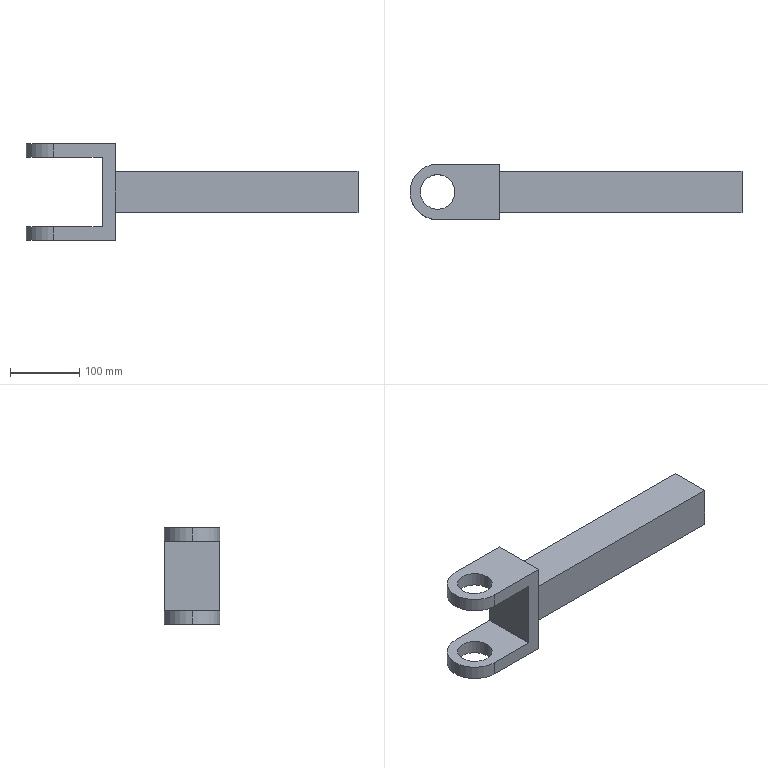Part | SolidWorks | 1 solid | 21 faces | box 480 x 80 x 140 mm | volume 1729991 mm3 | plane 13 | cylinder 8 | commonest cylinder face diameters 50 x4 80 x4
STEP:
#1=CARTESIAN_POINT('',(25.,0.,-50.));
#2=VERTEX_POINT('',#1);
#3=CARTESIAN_POINT('',(-25.,0.,-50.));
#4=VERTEX_POINT('',#3);
#5=CARTESIAN_POINT('',(0.,0.,-50.));
#6=DIRECTION('',(0.,0.,-1.));
#7=DIRECTION('',(-1.,0.,0.));
#8=AXIS2_PLACEMENT_3D('',#5,#6,#7);
#9=CIRCLE('',#8,25.);
#10=EDGE_CURVE('',#2,#4,#9,.T.);
#11=ORIENTED_EDGE('',*,*,#10,.F.);
#12=CARTESIAN_POINT('',(25.,0.,-70.));
#13=VERTEX_POINT('',#12);
#14=CARTESIAN_POINT('',(25.,0.,70.));
#15=DIRECTION('',(0.,0.,-1.));
#16=VECTOR('',#15,1000.);
#17=LINE('',#14,#16);
#18=EDGE_CURVE('',#2,#13,#17,.T.);
#19=ORIENTED_EDGE('',*,*,#18,.T.);
#20=CARTESIAN_POINT('',(-25.,0.,-70.));
#21=VERTEX_POINT('',#20);
#22=CARTESIAN_POINT('',(0.,0.,-70.));
#23=DIRECTION('',(0.,0.,1.));
#24=DIRECTION('',(1.,0.,0.));
#25=AXIS2_PLACEMENT_3D('',#22,#23,#24);
#26=CIRCLE('',#25,25.);
#27=EDGE_CURVE('',#21,#13,#26,.T.);
#28=ORIENTED_EDGE('',*,*,#27,.F.);
#29=CARTESIAN_POINT('',(-25.,0.,70.));
#30=DIRECTION('',(0.,0.,-1.));
#31=VECTOR('',#30,1000.);
#32=LINE('',#29,#31);
#33=EDGE_CURVE('',#4,#21,#32,.T.);
#34=ORIENTED_EDGE('',*,*,#33,.F.);
#35=EDGE_LOOP('',(#11,#19,#28,#34));
#36=FACE_OUTER_BOUND('',#35,.T.);
#37=CARTESIAN_POINT('',(0.,0.,70.));
#38=DIRECTION('',(0.,0.,-1.));
#39=DIRECTION('',(-1.,0.,0.));
#40=AXIS2_PLACEMENT_3D('',#37,#38,#39);
#41=CYLINDRICAL_SURFACE('',#40,25.);
#42=ADVANCED_FACE('',(#36),#41,.F.);
#43=CARTESIAN_POINT('',(0.,-40.,-50.));
#44=VERTEX_POINT('',#43);
#45=CARTESIAN_POINT('',(-40.,0.,-50.));
#46=VERTEX_POINT('',#45);
#47=CARTESIAN_POINT('',(0.,0.,-50.));
#48=DIRECTION('',(0.,0.,-1.));
#49=DIRECTION('',(-1.,0.,0.));
#50=AXIS2_PLACEMENT_3D('',#47,#48,#49);
#51=CIRCLE('',#50,40.);
#52=EDGE_CURVE('',#44,#46,#51,.T.);
#53=ORIENTED_EDGE('',*,*,#52,.T.);
#54=CARTESIAN_POINT('',(-40.,0.,-70.));
#55=VERTEX_POINT('',#54);
#56=CARTESIAN_POINT('',(-40.,0.,70.));
#57=DIRECTION('',(0.,0.,-1.));
#58=VECTOR('',#57,1000.);
#59=LINE('',#56,#58);
#60=EDGE_CURVE('',#46,#55,#59,.T.);
#61=ORIENTED_EDGE('',*,*,#60,.T.);
#62=CARTESIAN_POINT('',(0.,-40.,-70.));
#63=VERTEX_POINT('',#62);
#64=CARTESIAN_POINT('',(0.,0.,-70.));
#65=DIRECTION('',(0.,0.,1.));
#66=DIRECTION('',(1.,0.,0.));
#67=AXIS2_PLACEMENT_3D('',#64,#65,#66);
#68=CIRCLE('',#67,40.);
#69=EDGE_CURVE('',#55,#63,#68,.T.);
#70=ORIENTED_EDGE('',*,*,#69,.T.);
#71=CARTESIAN_POINT('',(0.,-40.,70.));
#72=DIRECTION('',(0.,0.,-1.));
#73=VECTOR('',#72,1000.);
#74=LINE('',#71,#73);
#75=EDGE_CURVE('',#44,#63,#74,.T.);
#76=ORIENTED_EDGE('',*,*,#75,.F.);
#77=EDGE_LOOP('',(#53,#61,#70,#76));
#78=FACE_OUTER_BOUND('',#77,.T.);
#79=CARTESIAN_POINT('',(0.,0.,70.));
#80=DIRECTION('',(0.,0.,-1.));
#81=DIRECTION('',(-1.,0.,0.));
#82=AXIS2_PLACEMENT_3D('',#79,#80,#81);
#83=CYLINDRICAL_SURFACE('',#82,40.);
#84=ADVANCED_FACE('',(#78),#83,.T.);
#85=CARTESIAN_POINT('',(-25.,0.,70.));
#86=VERTEX_POINT('',#85);
#87=CARTESIAN_POINT('',(25.,0.,70.));
#88=VERTEX_POINT('',#87);
#89=CARTESIAN_POINT('',(0.,0.,70.));
#90=DIRECTION('',(0.,0.,1.));
#91=DIRECTION('',(1.,0.,0.));
#92=AXIS2_PLACEMENT_3D('',#89,#90,#91);
#93=CIRCLE('',#92,25.);
#94=EDGE_CURVE('',#86,#88,#93,.T.);
#95=ORIENTED_EDGE('',*,*,#94,.T.);
#96=CARTESIAN_POINT('',(25.,0.,50.));
#97=VERTEX_POINT('',#96);
#98=CARTESIAN_POINT('',(25.,0.,70.));
#99=DIRECTION('',(0.,0.,-1.));
#100=VECTOR('',#99,1000.);
#101=LINE('',#98,#100);
#102=EDGE_CURVE('',#88,#97,#101,.T.);
#103=ORIENTED_EDGE('',*,*,#102,.T.);
#104=CARTESIAN_POINT('',(-25.,0.,50.));
#105=VERTEX_POINT('',#104);
#106=CARTESIAN_POINT('',(0.,0.,50.));
#107=DIRECTION('',(0.,0.,1.));
#108=DIRECTION('',(1.,0.,0.));
#109=AXIS2_PLACEMENT_3D('',#106,#107,#108);
#110=CIRCLE('',#109,25.);
#111=EDGE_CURVE('',#105,#97,#110,.T.);
#112=ORIENTED_EDGE('',*,*,#111,.F.);
#113=CARTESIAN_POINT('',(-25.,0.,70.));
#114=DIRECTION('',(0.,0.,-1.));
#115=VECTOR('',#114,1000.);
#116=LINE('',#113,#115);
#117=EDGE_CURVE('',#86,#105,#116,.T.);
#118=ORIENTED_EDGE('',*,*,#117,.F.);
#119=EDGE_LOOP('',(#95,#103,#112,#118));
#120=FACE_OUTER_BOUND('',#119,.T.);
#121=CARTESIAN_POINT('',(0.,0.,70.));
#122=DIRECTION('',(0.,0.,-1.));
#123=DIRECTION('',(-1.,0.,0.));
#124=AXIS2_PLACEMENT_3D('',#121,#122,#123);
#125=CYLINDRICAL_SURFACE('',#124,25.);
#126=ADVANCED_FACE('',(#120),#125,.F.);
#127=CARTESIAN_POINT('',(-40.,0.,70.));
#128=VERTEX_POINT('',#127);
#129=CARTESIAN_POINT('',(0.,-40.,70.));
#130=VERTEX_POINT('',#129);
#131=CARTESIAN_POINT('',(0.,0.,70.));
#132=DIRECTION('',(0.,0.,1.));
#133=DIRECTION('',(1.,0.,0.));
#134=AXIS2_PLACEMENT_3D('',#131,#132,#133);
#135=CIRCLE('',#134,40.);
#136=EDGE_CURVE('',#128,#130,#135,.T.);
#137=ORIENTED_EDGE('',*,*,#136,.F.);
#138=CARTESIAN_POINT('',(-40.,0.,50.));
#139=VERTEX_POINT('',#138);
#140=CARTESIAN_POINT('',(-40.,0.,70.));
#141=DIRECTION('',(0.,0.,-1.));
#142=VECTOR('',#141,1000.);
#143=LINE('',#140,#142);
#144=EDGE_CURVE('',#128,#139,#143,.T.);
#145=ORIENTED_EDGE('',*,*,#144,.T.);
#146=CARTESIAN_POINT('',(0.,-40.,50.));
#147=VERTEX_POINT('',#146);
#148=CARTESIAN_POINT('',(0.,0.,50.));
#149=DIRECTION('',(0.,0.,1.));
#150=DIRECTION('',(1.,0.,0.));
#151=AXIS2_PLACEMENT_3D('',#148,#149,#150);
#152=CIRCLE('',#151,40.);
#153=EDGE_CURVE('',#139,#147,#152,.T.);
#154=ORIENTED_EDGE('',*,*,#153,.T.);
#155=CARTESIAN_POINT('',(0.,-40.,70.));
#156=DIRECTION('',(0.,0.,-1.));
#157=VECTOR('',#156,1000.);
#158=LINE('',#155,#157);
#159=EDGE_CURVE('',#130,#147,#158,.T.);
#160=ORIENTED_EDGE('',*,*,#159,.F.);
#161=EDGE_LOOP('',(#137,#145,#154,#160));
#162=FACE_OUTER_BOUND('',#161,.T.);
#163=CARTESIAN_POINT('',(0.,0.,70.));
#164=DIRECTION('',(0.,0.,-1.));
#165=DIRECTION('',(-1.,0.,0.));
#166=AXIS2_PLACEMENT_3D('',#163,#164,#165);
#167=CYLINDRICAL_SURFACE('',#166,40.);
#168=ADVANCED_FACE('',(#162),#167,.T.);
#169=CARTESIAN_POINT('',(70.,-40.,-50.));
#170=VERTEX_POINT('',#169);
#171=CARTESIAN_POINT('',(70.,40.,-50.));
#172=VERTEX_POINT('',#171);
#173=CARTESIAN_POINT('',(70.,0.,-50.));
#174=DIRECTION('',(0.,1.,0.));
#175=VECTOR('',#174,1000.);
#176=LINE('',#173,#175);
#177=EDGE_CURVE('',#170,#172,#176,.T.);
#178=ORIENTED_EDGE('',*,*,#177,.F.);
#179=CARTESIAN_POINT('',(70.,-40.,50.));
#180=VERTEX_POINT('',#179);
#181=CARTESIAN_POINT('',(70.,-40.,70.));
#182=DIRECTION('',(0.,0.,-1.));
#183=VECTOR('',#182,1000.);
#184=LINE('',#181,#183);
#185=EDGE_CURVE('',#180,#170,#184,.T.);
#186=ORIENTED_EDGE('',*,*,#185,.F.);
#187=CARTESIAN_POINT('',(70.,40.,50.));
#188=VERTEX_POINT('',#187);
#189=CARTESIAN_POINT('',(70.,-100.,50.));
#190=DIRECTION('',(0.,1.,0.));
#191=VECTOR('',#190,1000.);
#192=LINE('',#189,#191);
#193=EDGE_CURVE('',#180,#188,#192,.T.);
#194=ORIENTED_EDGE('',*,*,#193,.T.);
#195=CARTESIAN_POINT('',(70.,40.,70.));
#196=DIRECTION('',(0.,0.,1.));
#197=VECTOR('',#196,1000.);
#198=LINE('',#195,#197);
#199=EDGE_CURVE('',#172,#188,#198,.T.);
#200=ORIENTED_EDGE('',*,*,#199,.F.);
#201=EDGE_LOOP('',(#178,#186,#194,#200));
#202=FACE_OUTER_BOUND('',#201,.T.);
#203=CARTESIAN_POINT('',(70.,0.,0.));
#204=DIRECTION('',(1.,0.,0.));
#205=DIRECTION('',(0.,0.,-1.));
#206=AXIS2_PLACEMENT_3D('',#203,#204,#205);
#207=PLANE('',#206);
#208=ADVANCED_FACE('',(#202),#207,.F.);
#209=ORIENTED_EDGE('',*,*,#111,.T.);
#210=CARTESIAN_POINT('',(0.,0.,50.));
#211=DIRECTION('',(0.,0.,1.));
#212=DIRECTION('',(1.,0.,0.));
#213=AXIS2_PLACEMENT_3D('',#210,#211,#212);
#214=CIRCLE('',#213,25.);
#215=EDGE_CURVE('',#97,#105,#214,.T.);
#216=ORIENTED_EDGE('',*,*,#215,.T.);
#217=EDGE_LOOP('',(#209,#216));
#218=FACE_BOUND('',#217,.T.);
#219=ORIENTED_EDGE('',*,*,#193,.F.);
#220=CARTESIAN_POINT('',(0.,-40.,50.));
#221=DIRECTION('',(1.,0.,0.));
#222=VECTOR('',#221,1000.);
#223=LINE('',#220,#222);
#224=EDGE_CURVE('',#147,#180,#223,.T.);
#225=ORIENTED_EDGE('',*,*,#224,.F.);
#226=ORIENTED_EDGE('',*,*,#153,.F.);
#227=CARTESIAN_POINT('',(0.,40.,50.));
#228=VERTEX_POINT('',#227);
#229=CARTESIAN_POINT('',(0.,0.,50.));
#230=DIRECTION('',(0.,0.,1.));
#231=DIRECTION('',(1.,0.,0.));
#232=AXIS2_PLACEMENT_3D('',#229,#230,#231);
#233=CIRCLE('',#232,40.);
#234=EDGE_CURVE('',#228,#139,#233,.T.);
#235=ORIENTED_EDGE('',*,*,#234,.F.);
#236=CARTESIAN_POINT('',(-80.,40.,50.));
#237=DIRECTION('',(1.,0.,0.));
#238=VECTOR('',#237,1000.);
#239=LINE('',#236,#238);
#240=EDGE_CURVE('',#228,#188,#239,.T.);
#241=ORIENTED_EDGE('',*,*,#240,.T.);
#242=EDGE_LOOP('',(#219,#225,#226,#235,#241));
#243=FACE_OUTER_BOUND('',#242,.T.);
#244=CARTESIAN_POINT('',(-80.,-100.,50.));
#245=DIRECTION('',(0.,0.,1.));
#246=DIRECTION('',(1.,0.,0.));
#247=AXIS2_PLACEMENT_3D('',#244,#245,#246);
#248=PLANE('',#247);
#249=ADVANCED_FACE('',(#218,#243),#248,.F.);
#250=ORIENTED_EDGE('',*,*,#75,.T.);
#251=CARTESIAN_POINT('',(90.,-40.,-70.));
#252=VERTEX_POINT('',#251);
#253=CARTESIAN_POINT('',(90.,-40.,-70.));
#254=DIRECTION('',(-1.,0.,0.));
#255=VECTOR('',#254,1000.);
#256=LINE('',#253,#255);
#257=EDGE_CURVE('',#252,#63,#256,.T.);
#258=ORIENTED_EDGE('',*,*,#257,.F.);
#259=CARTESIAN_POINT('',(90.,-40.,70.));
#260=VERTEX_POINT('',#259);
#261=CARTESIAN_POINT('',(90.,-40.,70.));
#262=DIRECTION('',(0.,0.,-1.));
#263=VECTOR('',#262,1000.);
#264=LINE('',#261,#263);
#265=EDGE_CURVE('',#260,#252,#264,.T.);
#266=ORIENTED_EDGE('',*,*,#265,.F.);
#267=CARTESIAN_POINT('',(0.,-40.,70.));
#268=DIRECTION('',(1.,0.,0.));
#269=VECTOR('',#268,1000.);
#270=LINE('',#267,#269);
#271=EDGE_CURVE('',#130,#260,#270,.T.);
#272=ORIENTED_EDGE('',*,*,#271,.F.);
#273=ORIENTED_EDGE('',*,*,#159,.T.);
#274=ORIENTED_EDGE('',*,*,#224,.T.);
#275=ORIENTED_EDGE('',*,*,#185,.T.);
#276=CARTESIAN_POINT('',(0.,-40.,-50.));
#277=DIRECTION('',(-1.,0.,0.));
#278=VECTOR('',#277,1000.);
#279=LINE('',#276,#278);
#280=EDGE_CURVE('',#170,#44,#279,.T.);
#281=ORIENTED_EDGE('',*,*,#280,.T.);
#282=EDGE_LOOP('',(#250,#258,#266,#272,#273,#274,#275,#281));
#283=FACE_OUTER_BOUND('',#282,.T.);
#284=CARTESIAN_POINT('',(0.,-40.,70.));
#285=DIRECTION('',(0.,1.,0.));
#286=DIRECTION('',(0.,0.,1.));
#287=AXIS2_PLACEMENT_3D('',#284,#285,#286);
#288=PLANE('',#287);
#289=ADVANCED_FACE('',(#283),#288,.F.);
#290=CARTESIAN_POINT('',(90.,40.,-70.));
#291=VERTEX_POINT('',#290);
#292=CARTESIAN_POINT('',(0.,40.,-70.));
#293=VERTEX_POINT('',#292);
#294=CARTESIAN_POINT('',(90.,40.,-70.));
#295=DIRECTION('',(-1.,0.,0.));
#296=VECTOR('',#295,1000.);
#297=LINE('',#294,#296);
#298=EDGE_CURVE('',#291,#293,#297,.T.);
#299=ORIENTED_EDGE('',*,*,#298,.T.);
#300=CARTESIAN_POINT('',(0.,40.,-50.));
#301=VERTEX_POINT('',#300);
#302=CARTESIAN_POINT('',(0.,40.,70.));
#303=DIRECTION('',(0.,0.,-1.));
#304=VECTOR('',#303,1000.);
#305=LINE('',#302,#304);
#306=EDGE_CURVE('',#301,#293,#305,.T.);
#307=ORIENTED_EDGE('',*,*,#306,.F.);
#308=CARTESIAN_POINT('',(-80.,40.,-50.));
#309=DIRECTION('',(-1.,0.,0.));
#310=VECTOR('',#309,1000.);
#311=LINE('',#308,#310);
#312=EDGE_CURVE('',#172,#301,#311,.T.);
#313=ORIENTED_EDGE('',*,*,#312,.F.);
#314=ORIENTED_EDGE('',*,*,#199,.T.);
#315=ORIENTED_EDGE('',*,*,#240,.F.);
#316=CARTESIAN_POINT('',(0.,40.,70.));
#317=VERTEX_POINT('',#316);
#318=CARTESIAN_POINT('',(0.,40.,70.));
#319=DIRECTION('',(0.,0.,-1.));
#320=VECTOR('',#319,1000.);
#321=LINE('',#318,#320);
#322=EDGE_CURVE('',#317,#228,#321,.T.);
#323=ORIENTED_EDGE('',*,*,#322,.F.);
#324=CARTESIAN_POINT('',(90.,40.,70.));
#325=VERTEX_POINT('',#324);
#326=CARTESIAN_POINT('',(0.,40.,70.));
#327=DIRECTION('',(1.,0.,0.));
#328=VECTOR('',#327,1000.);
#329=LINE('',#326,#328);
#330=EDGE_CURVE('',#317,#325,#329,.T.);
#331=ORIENTED_EDGE('',*,*,#330,.T.);
#332=CARTESIAN_POINT('',(90.,40.,70.));
#333=DIRECTION('',(0.,0.,1.));
#334=VECTOR('',#333,1000.);
#335=LINE('',#332,#334);
#336=EDGE_CURVE('',#291,#325,#335,.T.);
#337=ORIENTED_EDGE('',*,*,#336,.F.);
#338=EDGE_LOOP('',(#299,#307,#313,#314,#315,#323,#331,#337));
#339=FACE_OUTER_BOUND('',#338,.T.);
#340=CARTESIAN_POINT('',(0.,40.,70.));
#341=DIRECTION('',(0.,1.,0.));
#342=DIRECTION('',(0.,0.,1.));
#343=AXIS2_PLACEMENT_3D('',#340,#341,#342);
#344=PLANE('',#343);
#345=ADVANCED_FACE('',(#339),#344,.T.);
#346=ORIENTED_EDGE('',*,*,#144,.F.);
#347=CARTESIAN_POINT('',(0.,0.,70.));
#348=DIRECTION('',(0.,0.,1.));
#349=DIRECTION('',(1.,0.,0.));
#350=AXIS2_PLACEMENT_3D('',#347,#348,#349);
#351=CIRCLE('',#350,40.);
#352=EDGE_CURVE('',#317,#128,#351,.T.);
#353=ORIENTED_EDGE('',*,*,#352,.F.);
#354=ORIENTED_EDGE('',*,*,#322,.T.);
#355=ORIENTED_EDGE('',*,*,#234,.T.);
#356=EDGE_LOOP('',(#346,#353,#354,#355));
#357=FACE_OUTER_BOUND('',#356,.T.);
#358=CARTESIAN_POINT('',(0.,0.,70.));
#359=DIRECTION('',(0.,0.,-1.));
#360=DIRECTION('',(-1.,0.,0.));
#361=AXIS2_PLACEMENT_3D('',#358,#359,#360);
#362=CYLINDRICAL_SURFACE('',#361,40.);
#363=ADVANCED_FACE('',(#357),#362,.T.);
#364=ORIENTED_EDGE('',*,*,#102,.F.);
#365=CARTESIAN_POINT('',(0.,0.,70.));
#366=DIRECTION('',(0.,0.,1.));
#367=DIRECTION('',(1.,0.,0.));
#368=AXIS2_PLACEMENT_3D('',#365,#366,#367);
#369=CIRCLE('',#368,25.);
#370=EDGE_CURVE('',#88,#86,#369,.T.);
#371=ORIENTED_EDGE('',*,*,#370,.T.);
#372=ORIENTED_EDGE('',*,*,#117,.T.);
#373=ORIENTED_EDGE('',*,*,#215,.F.);
#374=EDGE_LOOP('',(#364,#371,#372,#373));
#375=FACE_OUTER_BOUND('',#374,.T.);
#376=CARTESIAN_POINT('',(0.,0.,70.));
#377=DIRECTION('',(0.,0.,-1.));
#378=DIRECTION('',(-1.,0.,0.));
#379=AXIS2_PLACEMENT_3D('',#376,#377,#378);
#380=CYLINDRICAL_SURFACE('',#379,25.);
#381=ADVANCED_FACE('',(#375),#380,.F.);
#382=CARTESIAN_POINT('',(90.,40.,70.));
#383=DIRECTION('',(0.,-1.,0.));
#384=VECTOR('',#383,1000.);
#385=LINE('',#382,#384);
#386=EDGE_CURVE('',#325,#260,#385,.T.);
#387=ORIENTED_EDGE('',*,*,#386,.F.);
#388=ORIENTED_EDGE('',*,*,#330,.F.);
#389=ORIENTED_EDGE('',*,*,#352,.T.);
#390=ORIENTED_EDGE('',*,*,#136,.T.);
#391=ORIENTED_EDGE('',*,*,#271,.T.);
#392=EDGE_LOOP('',(#387,#388,#389,#390,#391));
#393=FACE_OUTER_BOUND('',#392,.T.);
#394=ORIENTED_EDGE('',*,*,#94,.F.);
#395=ORIENTED_EDGE('',*,*,#370,.F.);
#396=EDGE_LOOP('',(#394,#395));
#397=FACE_BOUND('',#396,.T.);
#398=CARTESIAN_POINT('',(0.,0.,70.));
#399=DIRECTION('',(0.,0.,1.));
#400=DIRECTION('',(1.,0.,0.));
#401=AXIS2_PLACEMENT_3D('',#398,#399,#400);
#402=PLANE('',#401);
#403=ADVANCED_FACE('',(#393,#397),#402,.T.);
#404=ORIENTED_EDGE('',*,*,#257,.T.);
#405=ORIENTED_EDGE('',*,*,#69,.F.);
#406=CARTESIAN_POINT('',(0.,0.,-70.));
#407=DIRECTION('',(0.,0.,1.));
#408=DIRECTION('',(1.,0.,0.));
#409=AXIS2_PLACEMENT_3D('',#406,#407,#408);
#410=CIRCLE('',#409,40.);
#411=EDGE_CURVE('',#293,#55,#410,.T.);
#412=ORIENTED_EDGE('',*,*,#411,.F.);
#413=ORIENTED_EDGE('',*,*,#298,.F.);
#414=CARTESIAN_POINT('',(90.,40.,-70.));
#415=DIRECTION('',(0.,1.,0.));
#416=VECTOR('',#415,1000.);
#417=LINE('',#414,#416);
#418=EDGE_CURVE('',#252,#291,#417,.T.);
#419=ORIENTED_EDGE('',*,*,#418,.F.);
#420=EDGE_LOOP('',(#404,#405,#412,#413,#419));
#421=FACE_OUTER_BOUND('',#420,.T.);
#422=ORIENTED_EDGE('',*,*,#27,.T.);
#423=CARTESIAN_POINT('',(0.,0.,-70.));
#424=DIRECTION('',(0.,0.,1.));
#425=DIRECTION('',(1.,0.,0.));
#426=AXIS2_PLACEMENT_3D('',#423,#424,#425);
#427=CIRCLE('',#426,25.);
#428=EDGE_CURVE('',#13,#21,#427,.T.);
#429=ORIENTED_EDGE('',*,*,#428,.T.);
#430=EDGE_LOOP('',(#422,#429));
#431=FACE_BOUND('',#430,.T.);
#432=CARTESIAN_POINT('',(90.,40.,-70.));
#433=DIRECTION('',(0.,0.,1.));
#434=DIRECTION('',(1.,0.,0.));
#435=AXIS2_PLACEMENT_3D('',#432,#433,#434);
#436=PLANE('',#435);
#437=ADVANCED_FACE('',(#421,#431),#436,.F.);
#438=CARTESIAN_POINT('',(90.,-30.,-30.));
#439=VERTEX_POINT('',#438);
#440=CARTESIAN_POINT('',(90.,30.,-30.));
#441=VERTEX_POINT('',#440);
#442=CARTESIAN_POINT('',(90.,30.,-30.));
#443=DIRECTION('',(0.,1.,0.));
#444=VECTOR('',#443,1000.);
#445=LINE('',#442,#444);
#446=EDGE_CURVE('',#439,#441,#445,.T.);
#447=ORIENTED_EDGE('',*,*,#446,.F.);
#448=CARTESIAN_POINT('',(90.,-30.,30.));
#449=VERTEX_POINT('',#448);
#450=CARTESIAN_POINT('',(90.,-30.,30.));
#451=DIRECTION('',(0.,0.,-1.));
#452=VECTOR('',#451,1000.);
#453=LINE('',#450,#452);
#454=EDGE_CURVE('',#449,#439,#453,.T.);
#455=ORIENTED_EDGE('',*,*,#454,.F.);
#456=CARTESIAN_POINT('',(90.,30.,30.));
#457=VERTEX_POINT('',#456);
#458=CARTESIAN_POINT('',(90.,30.,30.));
#459=DIRECTION('',(0.,-1.,0.));
#460=VECTOR('',#459,1000.);
#461=LINE('',#458,#460);
#462=EDGE_CURVE('',#457,#449,#461,.T.);
#463=ORIENTED_EDGE('',*,*,#462,.F.);
#464=CARTESIAN_POINT('',(90.,30.,30.));
#465=DIRECTION('',(0.,0.,1.));
#466=VECTOR('',#465,1000.);
#467=LINE('',#464,#466);
#468=EDGE_CURVE('',#441,#457,#467,.T.);
#469=ORIENTED_EDGE('',*,*,#468,.F.);
#470=EDGE_LOOP('',(#447,#455,#463,#469));
#471=FACE_BOUND('',#470,.T.);
#472=ORIENTED_EDGE('',*,*,#418,.T.);
#473=ORIENTED_EDGE('',*,*,#336,.T.);
#474=ORIENTED_EDGE('',*,*,#386,.T.);
#475=ORIENTED_EDGE('',*,*,#265,.T.);
#476=EDGE_LOOP('',(#472,#473,#474,#475));
#477=FACE_OUTER_BOUND('',#476,.T.);
#478=CARTESIAN_POINT('',(90.,0.,0.));
#479=DIRECTION('',(1.,0.,0.));
#480=DIRECTION('',(0.,0.,-1.));
#481=AXIS2_PLACEMENT_3D('',#478,#479,#480);
#482=PLANE('',#481);
#483=ADVANCED_FACE('',(#471,#477),#482,.T.);
#484=CARTESIAN_POINT('',(0.,0.,-50.));
#485=DIRECTION('',(0.,0.,-1.));
#486=DIRECTION('',(-1.,0.,0.));
#487=AXIS2_PLACEMENT_3D('',#484,#485,#486);
#488=CIRCLE('',#487,25.);
#489=EDGE_CURVE('',#4,#2,#488,.T.);
#490=ORIENTED_EDGE('',*,*,#489,.T.);
#491=ORIENTED_EDGE('',*,*,#10,.T.);
#492=EDGE_LOOP('',(#490,#491));
#493=FACE_BOUND('',#492,.T.);
#494=ORIENTED_EDGE('',*,*,#280,.F.);
#495=ORIENTED_EDGE('',*,*,#177,.T.);
#496=ORIENTED_EDGE('',*,*,#312,.T.);
#497=CARTESIAN_POINT('',(0.,0.,-50.));
#498=DIRECTION('',(0.,0.,-1.));
#499=DIRECTION('',(-1.,0.,0.));
#500=AXIS2_PLACEMENT_3D('',#497,#498,#499);
#501=CIRCLE('',#500,40.);
#502=EDGE_CURVE('',#46,#301,#501,.T.);
#503=ORIENTED_EDGE('',*,*,#502,.F.);
#504=ORIENTED_EDGE('',*,*,#52,.F.);
#505=EDGE_LOOP('',(#494,#495,#496,#503,#504));
#506=FACE_OUTER_BOUND('',#505,.T.);
#507=CARTESIAN_POINT('',(-80.,-100.,-50.));
#508=DIRECTION('',(0.,0.,-1.));
#509=DIRECTION('',(-1.,0.,0.));
#510=AXIS2_PLACEMENT_3D('',#507,#508,#509);
#511=PLANE('',#510);
#512=ADVANCED_FACE('',(#493,#506),#511,.F.);
#513=ORIENTED_EDGE('',*,*,#60,.F.);
#514=ORIENTED_EDGE('',*,*,#502,.T.);
#515=ORIENTED_EDGE('',*,*,#306,.T.);
#516=ORIENTED_EDGE('',*,*,#411,.T.);
#517=EDGE_LOOP('',(#513,#514,#515,#516));
#518=FACE_OUTER_BOUND('',#517,.T.);
#519=CARTESIAN_POINT('',(0.,0.,70.));
#520=DIRECTION('',(0.,0.,-1.));
#521=DIRECTION('',(-1.,0.,0.));
#522=AXIS2_PLACEMENT_3D('',#519,#520,#521);
#523=CYLINDRICAL_SURFACE('',#522,40.);
#524=ADVANCED_FACE('',(#518),#523,.T.);
#525=ORIENTED_EDGE('',*,*,#18,.F.);
#526=ORIENTED_EDGE('',*,*,#489,.F.);
#527=ORIENTED_EDGE('',*,*,#33,.T.);
#528=ORIENTED_EDGE('',*,*,#428,.F.);
#529=EDGE_LOOP('',(#525,#526,#527,#528));
#530=FACE_OUTER_BOUND('',#529,.T.);
#531=CARTESIAN_POINT('',(0.,0.,70.));
#532=DIRECTION('',(0.,0.,-1.));
#533=DIRECTION('',(-1.,0.,0.));
#534=AXIS2_PLACEMENT_3D('',#531,#532,#533);
#535=CYLINDRICAL_SURFACE('',#534,25.);
#536=ADVANCED_FACE('',(#530),#535,.F.);
#537=ORIENTED_EDGE('',*,*,#446,.T.);
#538=CARTESIAN_POINT('',(440.,30.,-30.));
#539=VERTEX_POINT('',#538);
#540=CARTESIAN_POINT('',(440.,30.,-30.));
#541=DIRECTION('',(-1.,0.,0.));
#542=VECTOR('',#541,1000.);
#543=LINE('',#540,#542);
#544=EDGE_CURVE('',#539,#441,#543,.T.);
#545=ORIENTED_EDGE('',*,*,#544,.F.);
#546=CARTESIAN_POINT('',(440.,-30.,-30.));
#547=VERTEX_POINT('',#546);
#548=CARTESIAN_POINT('',(440.,30.,-30.));
#549=DIRECTION('',(0.,1.,0.));
#550=VECTOR('',#549,1000.);
#551=LINE('',#548,#550);
#552=EDGE_CURVE('',#547,#539,#551,.T.);
#553=ORIENTED_EDGE('',*,*,#552,.F.);
#554=CARTESIAN_POINT('',(440.,-30.,-30.));
#555=DIRECTION('',(-1.,0.,0.));
#556=VECTOR('',#555,1000.);
#557=LINE('',#554,#556);
#558=EDGE_CURVE('',#547,#439,#557,.T.);
#559=ORIENTED_EDGE('',*,*,#558,.T.);
#560=EDGE_LOOP('',(#537,#545,#553,#559));
#561=FACE_OUTER_BOUND('',#560,.T.);
#562=CARTESIAN_POINT('',(440.,30.,-30.));
#563=DIRECTION('',(0.,0.,1.));
#564=DIRECTION('',(1.,0.,0.));
#565=AXIS2_PLACEMENT_3D('',#562,#563,#564);
#566=PLANE('',#565);
#567=ADVANCED_FACE('',(#561),#566,.F.);
#568=ORIENTED_EDGE('',*,*,#468,.T.);
#569=CARTESIAN_POINT('',(440.,30.,30.));
#570=VERTEX_POINT('',#569);
#571=CARTESIAN_POINT('',(440.,30.,30.));
#572=DIRECTION('',(-1.,0.,0.));
#573=VECTOR('',#572,1000.);
#574=LINE('',#571,#573);
#575=EDGE_CURVE('',#570,#457,#574,.T.);
#576=ORIENTED_EDGE('',*,*,#575,.F.);
#577=CARTESIAN_POINT('',(440.,30.,30.));
#578=DIRECTION('',(0.,0.,1.));
#579=VECTOR('',#578,1000.);
#580=LINE('',#577,#579);
#581=EDGE_CURVE('',#539,#570,#580,.T.);
#582=ORIENTED_EDGE('',*,*,#581,.F.);
#583=ORIENTED_EDGE('',*,*,#544,.T.);
#584=EDGE_LOOP('',(#568,#576,#582,#583));
#585=FACE_OUTER_BOUND('',#584,.T.);
#586=CARTESIAN_POINT('',(440.,30.,30.));
#587=DIRECTION('',(0.,-1.,0.));
#588=DIRECTION('',(0.,0.,-1.));
#589=AXIS2_PLACEMENT_3D('',#586,#587,#588);
#590=PLANE('',#589);
#591=ADVANCED_FACE('',(#585),#590,.F.);
#592=ORIENTED_EDGE('',*,*,#462,.T.);
#593=CARTESIAN_POINT('',(440.,-30.,30.));
#594=VERTEX_POINT('',#593);
#595=CARTESIAN_POINT('',(440.,-30.,30.));
#596=DIRECTION('',(-1.,0.,0.));
#597=VECTOR('',#596,1000.);
#598=LINE('',#595,#597);
#599=EDGE_CURVE('',#594,#449,#598,.T.);
#600=ORIENTED_EDGE('',*,*,#599,.F.);
#601=CARTESIAN_POINT('',(440.,30.,30.));
#602=DIRECTION('',(0.,-1.,0.));
#603=VECTOR('',#602,1000.);
#604=LINE('',#601,#603);
#605=EDGE_CURVE('',#570,#594,#604,.T.);
#606=ORIENTED_EDGE('',*,*,#605,.F.);
#607=ORIENTED_EDGE('',*,*,#575,.T.);
#608=EDGE_LOOP('',(#592,#600,#606,#607));
#609=FACE_OUTER_BOUND('',#608,.T.);
#610=CARTESIAN_POINT('',(440.,30.,30.));
#611=DIRECTION('',(0.,0.,-1.));
#612=DIRECTION('',(-1.,0.,0.));
#613=AXIS2_PLACEMENT_3D('',#610,#611,#612);
#614=PLANE('',#613);
#615=ADVANCED_FACE('',(#609),#614,.F.);
#616=ORIENTED_EDGE('',*,*,#454,.T.);
#617=ORIENTED_EDGE('',*,*,#558,.F.);
#618=CARTESIAN_POINT('',(440.,-30.,30.));
#619=DIRECTION('',(0.,0.,-1.));
#620=VECTOR('',#619,1000.);
#621=LINE('',#618,#620);
#622=EDGE_CURVE('',#594,#547,#621,.T.);
#623=ORIENTED_EDGE('',*,*,#622,.F.);
#624=ORIENTED_EDGE('',*,*,#599,.T.);
#625=EDGE_LOOP('',(#616,#617,#623,#624));
#626=FACE_OUTER_BOUND('',#625,.T.);
#627=CARTESIAN_POINT('',(440.,-30.,30.));
#628=DIRECTION('',(0.,1.,0.));
#629=DIRECTION('',(0.,0.,1.));
#630=AXIS2_PLACEMENT_3D('',#627,#628,#629);
#631=PLANE('',#630);
#632=ADVANCED_FACE('',(#626),#631,.F.);
#633=ORIENTED_EDGE('',*,*,#552,.T.);
#634=ORIENTED_EDGE('',*,*,#581,.T.);
#635=ORIENTED_EDGE('',*,*,#605,.T.);
#636=ORIENTED_EDGE('',*,*,#622,.T.);
#637=EDGE_LOOP('',(#633,#634,#635,#636));
#638=FACE_OUTER_BOUND('',#637,.T.);
#639=CARTESIAN_POINT('',(440.,0.,0.));
#640=DIRECTION('',(1.,0.,0.));
#641=DIRECTION('',(0.,0.,-1.));
#642=AXIS2_PLACEMENT_3D('',#639,#640,#641);
#643=PLANE('',#642);
#644=ADVANCED_FACE('',(#638),#643,.T.);
#645=CLOSED_SHELL('',(#42,#84,#126,#168,#208,#249,#289,#345,#363,#381,#403,#437,#483,#512,#524,#536,#567,#591,#615,#632,#644));
#646=MANIFOLD_SOLID_BREP('',#645);
#647=CARTESIAN_POINT('',(0.,0.,0.));
#648=DIRECTION('',(0.,0.,1.));
#649=DIRECTION('',(1.,0.,0.));
#650=AXIS2_PLACEMENT_3D('',#647,#648,#649);
#651=(LENGTH_UNIT()NAMED_UNIT(*)SI_UNIT(.MILLI.,.METRE.));
#652=UNCERTAINTY_MEASURE_WITH_UNIT(LENGTH_MEASURE(0.00001),#651,'','');
#653=(NAMED_UNIT(*)PLANE_ANGLE_UNIT()SI_UNIT($,.RADIAN.));
#654=(NAMED_UNIT(*)SI_UNIT($,.STERADIAN.)SOLID_ANGLE_UNIT());
#655=(GEOMETRIC_REPRESENTATION_CONTEXT(3)GLOBAL_UNCERTAINTY_ASSIGNED_CONTEXT((#652))GLOBAL_UNIT_ASSIGNED_CONTEXT((#651,#653,#654))REPRESENTATION_CONTEXT('',''));
#656=ADVANCED_BREP_SHAPE_REPRESENTATION('',(#646,#650),#655);